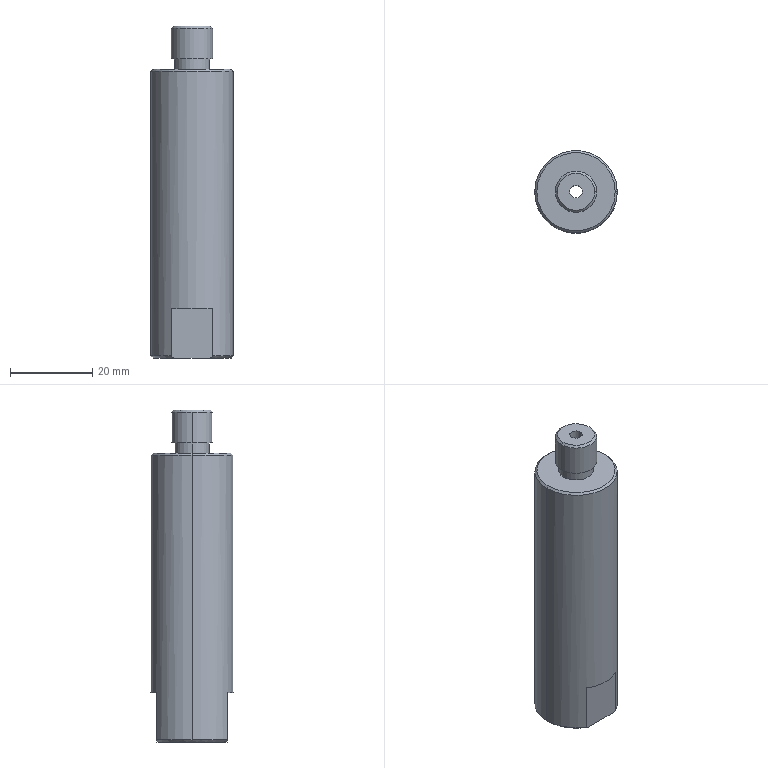Part | SolidWorks | features ICE 3, HoleWzd 2, Chamfer 1, Extrusion 1, MirrorPattern 1, RevCut 1 | 1 solid | 37 faces | box 20 x 20 x 80.5 mm | volume 19122 mm3 | plane 14 | cylinder 12 | cone 11 | commonest cylinder face diameters 3 x2 6 x2 8.5 x2 10 x2 11.125 x2 20 x2
STEP:
#1=CARTESIAN_POINT('',(4.5,0.,80.5));
#2=VERTEX_POINT('',#1);
#3=CARTESIAN_POINT('',(-4.5,0.,80.5));
#4=VERTEX_POINT('',#3);
#5=CARTESIAN_POINT('',(0.,0.,80.5));
#6=DIRECTION('',(0.,0.,1.));
#7=DIRECTION('',(1.,0.,0.));
#8=AXIS2_PLACEMENT_3D('',#5,#6,#7);
#9=CIRCLE('',#8,4.5);
#10=EDGE_CURVE('',#2,#4,#9,.T.);
#11=ORIENTED_EDGE('',*,*,#10,.F.);
#12=CARTESIAN_POINT('',(5.,0.,80.));
#13=VERTEX_POINT('',#12);
#14=CARTESIAN_POINT('',(4.5,0.,80.5));
#15=DIRECTION('',(0.7071,0.,-0.7071));
#16=VECTOR('',#15,1000.);
#17=LINE('',#14,#16);
#18=EDGE_CURVE('',#2,#13,#17,.T.);
#19=ORIENTED_EDGE('',*,*,#18,.T.);
#20=CARTESIAN_POINT('',(-5.,0.,80.));
#21=VERTEX_POINT('',#20);
#22=CARTESIAN_POINT('',(0.,0.,80.));
#23=DIRECTION('',(0.,0.,-1.));
#24=DIRECTION('',(1.,0.,0.));
#25=AXIS2_PLACEMENT_3D('',#22,#23,#24);
#26=CIRCLE('',#25,5.);
#27=EDGE_CURVE('',#21,#13,#26,.T.);
#28=ORIENTED_EDGE('',*,*,#27,.F.);
#29=CARTESIAN_POINT('',(-4.5,0.,80.5));
#30=DIRECTION('',(-0.7071,0.,-0.7071));
#31=VECTOR('',#30,1000.);
#32=LINE('',#29,#31);
#33=EDGE_CURVE('',#4,#21,#32,.T.);
#34=ORIENTED_EDGE('',*,*,#33,.F.);
#35=EDGE_LOOP('',(#11,#19,#28,#34));
#36=FACE_OUTER_BOUND('',#35,.T.);
#37=CARTESIAN_POINT('',(0.,0.,80.5));
#38=DIRECTION('',(0.,0.,-1.));
#39=DIRECTION('',(-1.,0.,0.));
#40=AXIS2_PLACEMENT_3D('',#37,#38,#39);
#41=CONICAL_SURFACE('',#40,4.5,0.7854);
#42=ADVANCED_FACE('',(#36),#41,.T.);
#43=CARTESIAN_POINT('',(9.5,0.,70.));
#44=VERTEX_POINT('',#43);
#45=CARTESIAN_POINT('',(-9.5,0.,70.));
#46=VERTEX_POINT('',#45);
#47=CARTESIAN_POINT('',(0.,0.,70.));
#48=DIRECTION('',(0.,0.,1.));
#49=DIRECTION('',(1.,0.,0.));
#50=AXIS2_PLACEMENT_3D('',#47,#48,#49);
#51=CIRCLE('',#50,9.5);
#52=EDGE_CURVE('',#44,#46,#51,.T.);
#53=ORIENTED_EDGE('',*,*,#52,.F.);
#54=CARTESIAN_POINT('',(10.,0.,69.5));
#55=VERTEX_POINT('',#54);
#56=CARTESIAN_POINT('',(9.5,0.,70.));
#57=DIRECTION('',(0.7071,0.,-0.7071));
#58=VECTOR('',#57,1000.);
#59=LINE('',#56,#58);
#60=EDGE_CURVE('',#44,#55,#59,.T.);
#61=ORIENTED_EDGE('',*,*,#60,.T.);
#62=CARTESIAN_POINT('',(-10.,0.,69.5));
#63=VERTEX_POINT('',#62);
#64=CARTESIAN_POINT('',(0.,0.,69.5));
#65=DIRECTION('',(0.,0.,-1.));
#66=DIRECTION('',(1.,0.,0.));
#67=AXIS2_PLACEMENT_3D('',#64,#65,#66);
#68=CIRCLE('',#67,10.);
#69=EDGE_CURVE('',#63,#55,#68,.T.);
#70=ORIENTED_EDGE('',*,*,#69,.F.);
#71=CARTESIAN_POINT('',(-9.5,0.,70.));
#72=DIRECTION('',(-0.7071,0.,-0.7071));
#73=VECTOR('',#72,1000.);
#74=LINE('',#71,#73);
#75=EDGE_CURVE('',#46,#63,#74,.T.);
#76=ORIENTED_EDGE('',*,*,#75,.F.);
#77=EDGE_LOOP('',(#53,#61,#70,#76));
#78=FACE_OUTER_BOUND('',#77,.T.);
#79=CARTESIAN_POINT('',(0.,0.,70.));
#80=DIRECTION('',(0.,0.,-1.));
#81=DIRECTION('',(-1.,0.,0.));
#82=AXIS2_PLACEMENT_3D('',#79,#80,#81);
#83=CONICAL_SURFACE('',#82,9.5,0.7854);
#84=ADVANCED_FACE('',(#78),#83,.T.);
#85=CARTESIAN_POINT('',(-3.,0.,18.61));
#86=VERTEX_POINT('',#85);
#87=CARTESIAN_POINT('',(3.,0.,18.61));
#88=VERTEX_POINT('',#87);
#89=CARTESIAN_POINT('',(0.,0.,18.61));
#90=DIRECTION('',(0.,0.,1.));
#91=DIRECTION('',(-1.,0.,0.));
#92=AXIS2_PLACEMENT_3D('',#89,#90,#91);
#93=CIRCLE('',#92,3.);
#94=EDGE_CURVE('',#86,#88,#93,.T.);
#95=ORIENTED_EDGE('',*,*,#94,.F.);
#96=CARTESIAN_POINT('',(-3.,0.,65.));
#97=VERTEX_POINT('',#96);
#98=CARTESIAN_POINT('',(-3.,0.,65.));
#99=DIRECTION('',(0.,0.,1.));
#100=VECTOR('',#99,1000.);
#101=LINE('',#98,#100);
#102=EDGE_CURVE('',#86,#97,#101,.T.);
#103=ORIENTED_EDGE('',*,*,#102,.T.);
#104=CARTESIAN_POINT('',(3.,0.,65.));
#105=VERTEX_POINT('',#104);
#106=CARTESIAN_POINT('',(0.,0.,65.));
#107=DIRECTION('',(0.,0.,1.));
#108=DIRECTION('',(1.,0.,0.));
#109=AXIS2_PLACEMENT_3D('',#106,#107,#108);
#110=CIRCLE('',#109,3.);
#111=EDGE_CURVE('',#97,#105,#110,.T.);
#112=ORIENTED_EDGE('',*,*,#111,.T.);
#113=CARTESIAN_POINT('',(3.,0.,65.));
#114=DIRECTION('',(0.,0.,1.));
#115=VECTOR('',#114,1000.);
#116=LINE('',#113,#115);
#117=EDGE_CURVE('',#88,#105,#116,.T.);
#118=ORIENTED_EDGE('',*,*,#117,.F.);
#119=EDGE_LOOP('',(#95,#103,#112,#118));
#120=FACE_OUTER_BOUND('',#119,.T.);
#121=CARTESIAN_POINT('',(0.,0.,65.));
#122=DIRECTION('',(0.,0.,1.));
#123=DIRECTION('',(1.,0.,0.));
#124=AXIS2_PLACEMENT_3D('',#121,#122,#123);
#125=CYLINDRICAL_SURFACE('',#124,3.);
#126=ADVANCED_FACE('',(#120),#125,.F.);
#127=CARTESIAN_POINT('',(5.944,0.,10.02));
#128=VERTEX_POINT('',#127);
#129=CARTESIAN_POINT('',(-5.944,0.,10.02));
#130=VERTEX_POINT('',#129);
#131=CARTESIAN_POINT('',(0.,0.,10.02));
#132=DIRECTION('',(0.,0.,-1.));
#133=DIRECTION('',(-1.,0.,0.));
#134=AXIS2_PLACEMENT_3D('',#131,#132,#133);
#135=CIRCLE('',#134,5.944);
#136=EDGE_CURVE('',#128,#130,#135,.T.);
#137=ORIENTED_EDGE('',*,*,#136,.F.);
#138=CARTESIAN_POINT('',(6.244,0.,0.));
#139=VERTEX_POINT('',#138);
#140=CARTESIAN_POINT('',(6.244,0.,0.));
#141=DIRECTION('',(0.02993,0.,-0.9996));
#142=VECTOR('',#141,1000.);
#143=LINE('',#140,#142);
#144=EDGE_CURVE('',#128,#139,#143,.T.);
#145=ORIENTED_EDGE('',*,*,#144,.T.);
#146=CARTESIAN_POINT('',(-6.244,0.,0.));
#147=VERTEX_POINT('',#146);
#148=CARTESIAN_POINT('',(0.,0.,0.));
#149=DIRECTION('',(0.,0.,-1.));
#150=DIRECTION('',(-1.,0.,0.));
#151=AXIS2_PLACEMENT_3D('',#148,#149,#150);
#152=CIRCLE('',#151,6.244);
#153=EDGE_CURVE('',#139,#147,#152,.T.);
#154=ORIENTED_EDGE('',*,*,#153,.T.);
#155=CARTESIAN_POINT('',(-6.244,0.,0.));
#156=DIRECTION('',(-0.02993,0.,-0.9996));
#157=VECTOR('',#156,1000.);
#158=LINE('',#155,#157);
#159=EDGE_CURVE('',#130,#147,#158,.T.);
#160=ORIENTED_EDGE('',*,*,#159,.F.);
#161=EDGE_LOOP('',(#137,#145,#154,#160));
#162=FACE_OUTER_BOUND('',#161,.T.);
#163=CARTESIAN_POINT('',(0.,0.,0.));
#164=DIRECTION('',(0.,0.,-1.));
#165=DIRECTION('',(-1.,0.,0.));
#166=AXIS2_PLACEMENT_3D('',#163,#164,#165);
#167=CONICAL_SURFACE('',#166,6.244,0.02993);
#168=ADVANCED_FACE('',(#162),#167,.F.);
#169=CARTESIAN_POINT('',(5.563,0.,17.07));
#170=VERTEX_POINT('',#169);
#171=CARTESIAN_POINT('',(-5.563,0.,17.07));
#172=VERTEX_POINT('',#171);
#173=CARTESIAN_POINT('',(0.,0.,17.07));
#174=DIRECTION('',(0.,0.,-1.));
#175=DIRECTION('',(-1.,0.,0.));
#176=AXIS2_PLACEMENT_3D('',#173,#174,#175);
#177=CIRCLE('',#176,5.563);
#178=EDGE_CURVE('',#170,#172,#177,.T.);
#179=ORIENTED_EDGE('',*,*,#178,.F.);
#180=CARTESIAN_POINT('',(5.563,0.,10.02));
#181=VERTEX_POINT('',#180);
#182=CARTESIAN_POINT('',(5.563,0.,0.));
#183=DIRECTION('',(0.,0.,-1.));
#184=VECTOR('',#183,1000.);
#185=LINE('',#182,#184);
#186=EDGE_CURVE('',#170,#181,#185,.T.);
#187=ORIENTED_EDGE('',*,*,#186,.T.);
#188=CARTESIAN_POINT('',(-5.563,0.,10.02));
#189=VERTEX_POINT('',#188);
#190=CARTESIAN_POINT('',(0.,0.,10.02));
#191=DIRECTION('',(0.,0.,-1.));
#192=DIRECTION('',(-1.,0.,0.));
#193=AXIS2_PLACEMENT_3D('',#190,#191,#192);
#194=CIRCLE('',#193,5.563);
#195=EDGE_CURVE('',#181,#189,#194,.T.);
#196=ORIENTED_EDGE('',*,*,#195,.T.);
#197=CARTESIAN_POINT('',(-5.563,0.,0.));
#198=DIRECTION('',(0.,0.,-1.));
#199=VECTOR('',#198,1000.);
#200=LINE('',#197,#199);
#201=EDGE_CURVE('',#172,#189,#200,.T.);
#202=ORIENTED_EDGE('',*,*,#201,.F.);
#203=EDGE_LOOP('',(#179,#187,#196,#202));
#204=FACE_OUTER_BOUND('',#203,.T.);
#205=CARTESIAN_POINT('',(0.,0.,0.));
#206=DIRECTION('',(0.,0.,-1.));
#207=DIRECTION('',(-1.,0.,0.));
#208=AXIS2_PLACEMENT_3D('',#205,#206,#207);
#209=CYLINDRICAL_SURFACE('',#208,5.563);
#210=ADVANCED_FACE('',(#204),#209,.F.);
#211=ORIENTED_EDGE('',*,*,#94,.T.);
#212=CARTESIAN_POINT('',(5.563,0.,17.07));
#213=DIRECTION('',(0.8572,0.,-0.515));
#214=VECTOR('',#213,1000.);
#215=LINE('',#212,#214);
#216=EDGE_CURVE('',#88,#170,#215,.T.);
#217=ORIENTED_EDGE('',*,*,#216,.T.);
#218=ORIENTED_EDGE('',*,*,#178,.T.);
#219=CARTESIAN_POINT('',(-5.563,0.,17.07));
#220=DIRECTION('',(-0.8572,0.,-0.515));
#221=VECTOR('',#220,1000.);
#222=LINE('',#219,#221);
#223=EDGE_CURVE('',#86,#172,#222,.T.);
#224=ORIENTED_EDGE('',*,*,#223,.F.);
#225=EDGE_LOOP('',(#211,#217,#218,#224));
#226=FACE_OUTER_BOUND('',#225,.T.);
#227=CARTESIAN_POINT('',(0.,0.,17.07));
#228=DIRECTION('',(0.,0.,-1.));
#229=DIRECTION('',(-1.,0.,0.));
#230=AXIS2_PLACEMENT_3D('',#227,#228,#229);
#231=CONICAL_SURFACE('',#230,5.563,1.03);
#232=ADVANCED_FACE('',(#226),#231,.F.);
#233=CARTESIAN_POINT('',(1.5,0.,65.));
#234=VERTEX_POINT('',#233);
#235=CARTESIAN_POINT('',(-1.5,0.,65.));
#236=VERTEX_POINT('',#235);
#237=CARTESIAN_POINT('',(0.,0.,65.));
#238=DIRECTION('',(0.,0.,-1.));
#239=DIRECTION('',(1.,0.,0.));
#240=AXIS2_PLACEMENT_3D('',#237,#238,#239);
#241=CIRCLE('',#240,1.5);
#242=EDGE_CURVE('',#234,#236,#241,.T.);
#243=ORIENTED_EDGE('',*,*,#242,.T.);
#244=CARTESIAN_POINT('',(-1.5,0.,80.5));
#245=VERTEX_POINT('',#244);
#246=CARTESIAN_POINT('',(-1.5,0.,65.));
#247=DIRECTION('',(0.,0.,1.));
#248=VECTOR('',#247,1000.);
#249=LINE('',#246,#248);
#250=EDGE_CURVE('',#236,#245,#249,.T.);
#251=ORIENTED_EDGE('',*,*,#250,.T.);
#252=CARTESIAN_POINT('',(1.5,0.,80.5));
#253=VERTEX_POINT('',#252);
#254=CARTESIAN_POINT('',(0.,0.,80.5));
#255=DIRECTION('',(0.,0.,1.));
#256=DIRECTION('',(1.,0.,0.));
#257=AXIS2_PLACEMENT_3D('',#254,#255,#256);
#258=CIRCLE('',#257,1.5);
#259=EDGE_CURVE('',#245,#253,#258,.T.);
#260=ORIENTED_EDGE('',*,*,#259,.T.);
#261=CARTESIAN_POINT('',(1.5,0.,65.));
#262=DIRECTION('',(0.,0.,1.));
#263=VECTOR('',#262,1000.);
#264=LINE('',#261,#263);
#265=EDGE_CURVE('',#234,#253,#264,.T.);
#266=ORIENTED_EDGE('',*,*,#265,.F.);
#267=EDGE_LOOP('',(#243,#251,#260,#266));
#268=FACE_OUTER_BOUND('',#267,.T.);
#269=CARTESIAN_POINT('',(0.,0.,65.));
#270=DIRECTION('',(0.,0.,1.));
#271=DIRECTION('',(1.,0.,0.));
#272=AXIS2_PLACEMENT_3D('',#269,#270,#271);
#273=CYLINDRICAL_SURFACE('',#272,1.5);
#274=ADVANCED_FACE('',(#268),#273,.F.);
#275=ORIENTED_EDGE('',*,*,#27,.T.);
#276=CARTESIAN_POINT('',(5.,0.,72.5));
#277=VERTEX_POINT('',#276);
#278=CARTESIAN_POINT('',(5.,0.,80.5));
#279=DIRECTION('',(0.,0.,-1.));
#280=VECTOR('',#279,1000.);
#281=LINE('',#278,#280);
#282=EDGE_CURVE('',#13,#277,#281,.T.);
#283=ORIENTED_EDGE('',*,*,#282,.T.);
#284=CARTESIAN_POINT('',(-5.,0.,72.5));
#285=VERTEX_POINT('',#284);
#286=CARTESIAN_POINT('',(0.,0.,72.5));
#287=DIRECTION('',(0.,0.,1.));
#288=DIRECTION('',(1.,0.,0.));
#289=AXIS2_PLACEMENT_3D('',#286,#287,#288);
#290=CIRCLE('',#289,5.);
#291=EDGE_CURVE('',#277,#285,#290,.T.);
#292=ORIENTED_EDGE('',*,*,#291,.T.);
#293=CARTESIAN_POINT('',(-5.,0.,80.5));
#294=DIRECTION('',(0.,0.,-1.));
#295=VECTOR('',#294,1000.);
#296=LINE('',#293,#295);
#297=EDGE_CURVE('',#21,#285,#296,.T.);
#298=ORIENTED_EDGE('',*,*,#297,.F.);
#299=EDGE_LOOP('',(#275,#283,#292,#298));
#300=FACE_OUTER_BOUND('',#299,.T.);
#301=CARTESIAN_POINT('',(0.,0.,80.5));
#302=DIRECTION('',(0.,0.,-1.));
#303=DIRECTION('',(-1.,0.,0.));
#304=AXIS2_PLACEMENT_3D('',#301,#302,#303);
#305=CYLINDRICAL_SURFACE('',#304,5.);
#306=ADVANCED_FACE('',(#300),#305,.T.);
#307=CARTESIAN_POINT('',(4.25,0.,70.));
#308=VERTEX_POINT('',#307);
#309=CARTESIAN_POINT('',(-4.25,0.,70.));
#310=VERTEX_POINT('',#309);
#311=CARTESIAN_POINT('',(0.,0.,70.));
#312=DIRECTION('',(0.,0.,1.));
#313=DIRECTION('',(1.,0.,0.));
#314=AXIS2_PLACEMENT_3D('',#311,#312,#313);
#315=CIRCLE('',#314,4.25);
#316=EDGE_CURVE('',#308,#310,#315,.T.);
#317=ORIENTED_EDGE('',*,*,#316,.T.);
#318=CARTESIAN_POINT('',(-4.25,0.,72.5));
#319=VERTEX_POINT('',#318);
#320=CARTESIAN_POINT('',(-4.25,0.,80.5));
#321=DIRECTION('',(0.,0.,1.));
#322=VECTOR('',#321,1000.);
#323=LINE('',#320,#322);
#324=EDGE_CURVE('',#310,#319,#323,.T.);
#325=ORIENTED_EDGE('',*,*,#324,.T.);
#326=CARTESIAN_POINT('',(4.25,0.,72.5));
#327=VERTEX_POINT('',#326);
#328=CARTESIAN_POINT('',(0.,0.,72.5));
#329=DIRECTION('',(0.,0.,1.));
#330=DIRECTION('',(1.,0.,0.));
#331=AXIS2_PLACEMENT_3D('',#328,#329,#330);
#332=CIRCLE('',#331,4.25);
#333=EDGE_CURVE('',#327,#319,#332,.T.);
#334=ORIENTED_EDGE('',*,*,#333,.F.);
#335=CARTESIAN_POINT('',(4.25,0.,80.5));
#336=DIRECTION('',(0.,0.,1.));
#337=VECTOR('',#336,1000.);
#338=LINE('',#335,#337);
#339=EDGE_CURVE('',#308,#327,#338,.T.);
#340=ORIENTED_EDGE('',*,*,#339,.F.);
#341=EDGE_LOOP('',(#317,#325,#334,#340));
#342=FACE_OUTER_BOUND('',#341,.T.);
#343=CARTESIAN_POINT('',(0.,0.,80.5));
#344=DIRECTION('',(0.,0.,1.));
#345=DIRECTION('',(1.,0.,0.));
#346=AXIS2_PLACEMENT_3D('',#343,#344,#345);
#347=CYLINDRICAL_SURFACE('',#346,4.25);
#348=ADVANCED_FACE('',(#342),#347,.T.);
#349=CARTESIAN_POINT('',(9.5,0.,0.));
#350=VERTEX_POINT('',#349);
#351=CARTESIAN_POINT('',(4.243,-8.5,0.));
#352=VERTEX_POINT('',#351);
#353=CARTESIAN_POINT('',(0.,0.,0.));
#354=DIRECTION('',(0.,0.,-1.));
#355=DIRECTION('',(1.,0.,0.));
#356=AXIS2_PLACEMENT_3D('',#353,#354,#355);
#357=CIRCLE('',#356,9.5);
#358=EDGE_CURVE('',#350,#352,#357,.T.);
#359=ORIENTED_EDGE('',*,*,#358,.F.);
#360=CARTESIAN_POINT('',(10.,0.,0.5));
#361=VERTEX_POINT('',#360);
#362=CARTESIAN_POINT('',(10.,0.,0.5));
#363=DIRECTION('',(0.7071,0.,0.7071));
#364=VECTOR('',#363,1000.);
#365=LINE('',#362,#364);
#366=EDGE_CURVE('',#350,#361,#365,.T.);
#367=ORIENTED_EDGE('',*,*,#366,.T.);
#368=CARTESIAN_POINT('',(5.,-8.66,0.5));
#369=VERTEX_POINT('',#368);
#370=CARTESIAN_POINT('',(0.,0.,0.5));
#371=DIRECTION('',(0.,0.,1.));
#372=DIRECTION('',(1.,0.,0.));
#373=AXIS2_PLACEMENT_3D('',#370,#371,#372);
#374=CIRCLE('',#373,10.);
#375=EDGE_CURVE('',#369,#361,#374,.T.);
#376=ORIENTED_EDGE('',*,*,#375,.F.);
#377=CARTESIAN_POINT('',(5.,-8.5,0.3615));
#378=VERTEX_POINT('',#377);
#379=CARTESIAN_POINT('',(5.,-8.66,0.5));
#380=CARTESIAN_POINT('',(5.,-8.607,0.4538));
#381=CARTESIAN_POINT('',(5.,-8.553,0.4076));
#382=CARTESIAN_POINT('',(5.,-8.5,0.3615));
#383=B_SPLINE_CURVE_WITH_KNOTS('',3,(#379,#380,#381,#382),.UNSPECIFIED.,.F.,.F.,(4,4),(0.002946,0.003158),.UNSPECIFIED.);
#384=EDGE_CURVE('',#369,#378,#383,.T.);
#385=ORIENTED_EDGE('',*,*,#384,.T.);
#386=CARTESIAN_POINT('',(5.,-8.5,0.3615));
#387=CARTESIAN_POINT('',(4.751,-8.5,0.2351));
#388=CARTESIAN_POINT('',(4.498,-8.5,0.1139));
#389=CARTESIAN_POINT('',(4.243,-8.5,0.));
#390=B_SPLINE_CURVE_WITH_KNOTS('',3,(#386,#387,#388,#389),.UNSPECIFIED.,.F.,.F.,(4,4),(0.007243,0.008076),.UNSPECIFIED.);
#391=EDGE_CURVE('',#378,#352,#390,.T.);
#392=ORIENTED_EDGE('',*,*,#391,.T.);
#393=EDGE_LOOP('',(#359,#367,#376,#385,#392));
#394=FACE_OUTER_BOUND('',#393,.T.);
#395=CARTESIAN_POINT('',(0.,0.,0.5));
#396=DIRECTION('',(0.,0.,1.));
#397=DIRECTION('',(1.,0.,0.));
#398=AXIS2_PLACEMENT_3D('',#395,#396,#397);
#399=CONICAL_SURFACE('',#398,10.,0.7854);
#400=ADVANCED_FACE('',(#394),#399,.T.);
#401=ORIENTED_EDGE('',*,*,#69,.T.);
#402=CARTESIAN_POINT('',(10.,0.,70.));
#403=DIRECTION('',(0.,0.,-1.));
#404=VECTOR('',#403,1000.);
#405=LINE('',#402,#404);
#406=EDGE_CURVE('',#55,#361,#405,.T.);
#407=ORIENTED_EDGE('',*,*,#406,.T.);
#408=CARTESIAN_POINT('',(5.,8.66,0.5));
#409=VERTEX_POINT('',#408);
#410=CARTESIAN_POINT('',(0.,0.,0.5));
#411=DIRECTION('',(0.,0.,1.));
#412=DIRECTION('',(1.,0.,0.));
#413=AXIS2_PLACEMENT_3D('',#410,#411,#412);
#414=CIRCLE('',#413,10.);
#415=EDGE_CURVE('',#361,#409,#414,.T.);
#416=ORIENTED_EDGE('',*,*,#415,.T.);
#417=CARTESIAN_POINT('',(5.,8.66,12.));
#418=VERTEX_POINT('',#417);
#419=CARTESIAN_POINT('',(5.,8.66,70.));
#420=DIRECTION('',(0.,0.,1.));
#421=VECTOR('',#420,1000.);
#422=LINE('',#419,#421);
#423=EDGE_CURVE('',#409,#418,#422,.T.);
#424=ORIENTED_EDGE('',*,*,#423,.T.);
#425=CARTESIAN_POINT('',(-5.,8.66,12.));
#426=VERTEX_POINT('',#425);
#427=CARTESIAN_POINT('',(0.,0.,12.));
#428=DIRECTION('',(0.,0.,1.));
#429=DIRECTION('',(1.,0.,0.));
#430=AXIS2_PLACEMENT_3D('',#427,#428,#429);
#431=CIRCLE('',#430,10.);
#432=EDGE_CURVE('',#418,#426,#431,.T.);
#433=ORIENTED_EDGE('',*,*,#432,.T.);
#434=CARTESIAN_POINT('',(-5.,8.66,0.5));
#435=VERTEX_POINT('',#434);
#436=CARTESIAN_POINT('',(-5.,8.66,70.));
#437=DIRECTION('',(0.,0.,-1.));
#438=VECTOR('',#437,1000.);
#439=LINE('',#436,#438);
#440=EDGE_CURVE('',#426,#435,#439,.T.);
#441=ORIENTED_EDGE('',*,*,#440,.T.);
#442=CARTESIAN_POINT('',(-10.,0.,0.5));
#443=VERTEX_POINT('',#442);
#444=CARTESIAN_POINT('',(0.,0.,0.5));
#445=DIRECTION('',(0.,0.,1.));
#446=DIRECTION('',(1.,0.,0.));
#447=AXIS2_PLACEMENT_3D('',#444,#445,#446);
#448=CIRCLE('',#447,10.);
#449=EDGE_CURVE('',#435,#443,#448,.T.);
#450=ORIENTED_EDGE('',*,*,#449,.T.);
#451=CARTESIAN_POINT('',(-10.,0.,70.));
#452=DIRECTION('',(0.,0.,-1.));
#453=VECTOR('',#452,1000.);
#454=LINE('',#451,#453);
#455=EDGE_CURVE('',#63,#443,#454,.T.);
#456=ORIENTED_EDGE('',*,*,#455,.F.);
#457=EDGE_LOOP('',(#401,#407,#416,#424,#433,#441,#450,#456));
#458=FACE_OUTER_BOUND('',#457,.T.);
#459=CARTESIAN_POINT('',(0.,0.,70.));
#460=DIRECTION('',(0.,0.,-1.));
#461=DIRECTION('',(-1.,0.,0.));
#462=AXIS2_PLACEMENT_3D('',#459,#460,#461);
#463=CYLINDRICAL_SURFACE('',#462,10.);
#464=ADVANCED_FACE('',(#458),#463,.T.);
#465=CARTESIAN_POINT('',(0.,0.,0.));
#466=DIRECTION('',(0.,0.,-1.));
#467=DIRECTION('',(-1.,0.,0.));
#468=AXIS2_PLACEMENT_3D('',#465,#466,#467);
#469=CIRCLE('',#468,6.244);
#470=EDGE_CURVE('',#147,#139,#469,.T.);
#471=ORIENTED_EDGE('',*,*,#470,.F.);
#472=ORIENTED_EDGE('',*,*,#153,.F.);
#473=EDGE_LOOP('',(#471,#472));
#474=FACE_BOUND('',#473,.T.);
#475=CARTESIAN_POINT('',(-4.243,-8.5,0.));
#476=VERTEX_POINT('',#475);
#477=CARTESIAN_POINT('',(-5.,-8.5,0.));
#478=DIRECTION('',(-1.,0.,0.));
#479=VECTOR('',#478,1000.);
#480=LINE('',#477,#479);
#481=EDGE_CURVE('',#352,#476,#480,.T.);
#482=ORIENTED_EDGE('',*,*,#481,.T.);
#483=CARTESIAN_POINT('',(-4.243,8.5,0.));
#484=VERTEX_POINT('',#483);
#485=CARTESIAN_POINT('',(0.,0.,0.));
#486=DIRECTION('',(0.,0.,-1.));
#487=DIRECTION('',(1.,0.,0.));
#488=AXIS2_PLACEMENT_3D('',#485,#486,#487);
#489=CIRCLE('',#488,9.5);
#490=EDGE_CURVE('',#476,#484,#489,.T.);
#491=ORIENTED_EDGE('',*,*,#490,.T.);
#492=CARTESIAN_POINT('',(4.243,8.5,0.));
#493=VERTEX_POINT('',#492);
#494=CARTESIAN_POINT('',(-5.,8.5,0.));
#495=DIRECTION('',(-1.,0.,0.));
#496=VECTOR('',#495,1000.);
#497=LINE('',#494,#496);
#498=EDGE_CURVE('',#493,#484,#497,.T.);
#499=ORIENTED_EDGE('',*,*,#498,.F.);
#500=CARTESIAN_POINT('',(0.,0.,0.));
#501=DIRECTION('',(0.,0.,-1.));
#502=DIRECTION('',(1.,0.,0.));
#503=AXIS2_PLACEMENT_3D('',#500,#501,#502);
#504=CIRCLE('',#503,9.5);
#505=EDGE_CURVE('',#493,#350,#504,.T.);
#506=ORIENTED_EDGE('',*,*,#505,.T.);
#507=ORIENTED_EDGE('',*,*,#358,.T.);
#508=EDGE_LOOP('',(#482,#491,#499,#506,#507));
#509=FACE_OUTER_BOUND('',#508,.T.);
#510=CARTESIAN_POINT('',(0.,0.,0.));
#511=DIRECTION('',(0.,0.,1.));
#512=DIRECTION('',(1.,0.,0.));
#513=AXIS2_PLACEMENT_3D('',#510,#511,#512);
#514=PLANE('',#513);
#515=ADVANCED_FACE('',(#474,#509),#514,.F.);
#516=ORIENTED_EDGE('',*,*,#406,.F.);
#517=CARTESIAN_POINT('',(0.,0.,69.5));
#518=DIRECTION('',(0.,0.,-1.));
#519=DIRECTION('',(1.,0.,0.));
#520=AXIS2_PLACEMENT_3D('',#517,#518,#519);
#521=CIRCLE('',#520,10.);
#522=EDGE_CURVE('',#55,#63,#521,.T.);
#523=ORIENTED_EDGE('',*,*,#522,.T.);
#524=ORIENTED_EDGE('',*,*,#455,.T.);
#525=CARTESIAN_POINT('',(-5.,-8.66,0.5));
#526=VERTEX_POINT('',#525);
#527=CARTESIAN_POINT('',(0.,0.,0.5));
#528=DIRECTION('',(0.,0.,1.));
#529=DIRECTION('',(1.,0.,0.));
#530=AXIS2_PLACEMENT_3D('',#527,#528,#529);
#531=CIRCLE('',#530,10.);
#532=EDGE_CURVE('',#443,#526,#531,.T.);
#533=ORIENTED_EDGE('',*,*,#532,.T.);
#534=CARTESIAN_POINT('',(-5.,-8.66,12.));
#535=VERTEX_POINT('',#534);
#536=CARTESIAN_POINT('',(-5.,-8.66,70.));
#537=DIRECTION('',(0.,0.,-1.));
#538=VECTOR('',#537,1000.);
#539=LINE('',#536,#538);
#540=EDGE_CURVE('',#535,#526,#539,.T.);
#541=ORIENTED_EDGE('',*,*,#540,.F.);
#542=CARTESIAN_POINT('',(5.,-8.66,12.));
#543=VERTEX_POINT('',#542);
#544=CARTESIAN_POINT('',(0.,0.,12.));
#545=DIRECTION('',(0.,0.,-1.));
#546=DIRECTION('',(-1.,0.,0.));
#547=AXIS2_PLACEMENT_3D('',#544,#545,#546);
#548=CIRCLE('',#547,10.);
#549=EDGE_CURVE('',#543,#535,#548,.T.);
#550=ORIENTED_EDGE('',*,*,#549,.F.);
#551=CARTESIAN_POINT('',(5.,-8.66,70.));
#552=DIRECTION('',(0.,0.,1.));
#553=VECTOR('',#552,1000.);
#554=LINE('',#551,#553);
#555=EDGE_CURVE('',#369,#543,#554,.T.);
#556=ORIENTED_EDGE('',*,*,#555,.F.);
#557=ORIENTED_EDGE('',*,*,#375,.T.);
#558=EDGE_LOOP('',(#516,#523,#524,#533,#541,#550,#556,#557));
#559=FACE_OUTER_BOUND('',#558,.T.);
#560=CARTESIAN_POINT('',(0.,0.,70.));
#561=DIRECTION('',(0.,0.,-1.));
#562=DIRECTION('',(-1.,0.,0.));
#563=AXIS2_PLACEMENT_3D('',#560,#561,#562);
#564=CYLINDRICAL_SURFACE('',#563,10.);
#565=ADVANCED_FACE('',(#559),#564,.T.);
#566=ORIENTED_EDGE('',*,*,#366,.F.);
#567=ORIENTED_EDGE('',*,*,#505,.F.);
#568=CARTESIAN_POINT('',(5.,8.5,0.3615));
#569=VERTEX_POINT('',#568);
#570=CARTESIAN_POINT('',(4.243,8.5,0.));
#571=CARTESIAN_POINT('',(4.498,8.5,0.114));
#572=CARTESIAN_POINT('',(4.75,8.5,0.2349));
#573=CARTESIAN_POINT('',(5.,8.5,0.3615));
#574=B_SPLINE_CURVE_WITH_KNOTS('',3,(#570,#571,#572,#573),.UNSPECIFIED.,.F.,.F.,(4,4),(0.01684,0.01768),.UNSPECIFIED.);
#575=EDGE_CURVE('',#493,#569,#574,.T.);
#576=ORIENTED_EDGE('',*,*,#575,.T.);
#577=CARTESIAN_POINT('',(5.,8.66,0.5));
#578=CARTESIAN_POINT('',(5.,8.607,0.4538));
#579=CARTESIAN_POINT('',(5.,8.553,0.4076));
#580=CARTESIAN_POINT('',(5.,8.5,0.3615));
#581=B_SPLINE_CURVE_WITH_KNOTS('',3,(#577,#578,#579,#580),.UNSPECIFIED.,.F.,.F.,(4,4),(0.002946,0.003158),.UNSPECIFIED.);
#582=EDGE_CURVE('',#409,#569,#581,.T.);
#583=ORIENTED_EDGE('',*,*,#582,.F.);
#584=ORIENTED_EDGE('',*,*,#415,.F.);
#585=EDGE_LOOP('',(#566,#567,#576,#583,#584));
#586=FACE_OUTER_BOUND('',#585,.T.);
#587=CARTESIAN_POINT('',(0.,0.,0.5));
#588=DIRECTION('',(0.,0.,1.));
#589=DIRECTION('',(1.,0.,0.));
#590=AXIS2_PLACEMENT_3D('',#587,#588,#589);
#591=CONICAL_SURFACE('',#590,10.,0.7854);
#592=ADVANCED_FACE('',(#586),#591,.T.);
#593=CARTESIAN_POINT('',(-5.,-8.5,0.3615));
#594=VERTEX_POINT('',#593);
#595=CARTESIAN_POINT('',(-4.243,-8.5,0.));
#596=CARTESIAN_POINT('',(-4.498,-8.5,0.114));
#597=CARTESIAN_POINT('',(-4.75,-8.5,0.2349));
#598=CARTESIAN_POINT('',(-5.,-8.5,0.3615));
#599=B_SPLINE_CURVE_WITH_KNOTS('',3,(#595,#596,#597,#598),.UNSPECIFIED.,.F.,.F.,(4,4),(0.01684,0.01768),.UNSPECIFIED.);
#600=EDGE_CURVE('',#476,#594,#599,.T.);
#601=ORIENTED_EDGE('',*,*,#600,.T.);
#602=CARTESIAN_POINT('',(-5.,-8.5,0.3615));
#603=CARTESIAN_POINT('',(-5.,-8.553,0.4076));
#604=CARTESIAN_POINT('',(-5.,-8.607,0.4538));
#605=CARTESIAN_POINT('',(-5.,-8.66,0.5));
#606=B_SPLINE_CURVE_WITH_KNOTS('',3,(#602,#603,#604,#605),.UNSPECIFIED.,.F.,.F.,(4,4),(0.003021,0.003233),.UNSPECIFIED.);
#607=EDGE_CURVE('',#594,#526,#606,.T.);
#608=ORIENTED_EDGE('',*,*,#607,.T.);
#609=ORIENTED_EDGE('',*,*,#532,.F.);
#610=ORIENTED_EDGE('',*,*,#449,.F.);
#611=CARTESIAN_POINT('',(-5.,8.5,0.3615));
#612=VERTEX_POINT('',#611);
#613=CARTESIAN_POINT('',(-5.,8.5,0.3615));
#614=CARTESIAN_POINT('',(-5.,8.553,0.4076));
#615=CARTESIAN_POINT('',(-5.,8.607,0.4538));
#616=CARTESIAN_POINT('',(-5.,8.66,0.5));
#617=B_SPLINE_CURVE_WITH_KNOTS('',3,(#613,#614,#615,#616),.UNSPECIFIED.,.F.,.F.,(4,4),(0.003021,0.003233),.UNSPECIFIED.);
#618=EDGE_CURVE('',#612,#435,#617,.T.);
#619=ORIENTED_EDGE('',*,*,#618,.F.);
#620=CARTESIAN_POINT('',(-5.,8.5,0.3615));
#621=CARTESIAN_POINT('',(-4.751,8.5,0.2351));
#622=CARTESIAN_POINT('',(-4.498,8.5,0.1139));
#623=CARTESIAN_POINT('',(-4.243,8.5,0.));
#624=B_SPLINE_CURVE_WITH_KNOTS('',3,(#620,#621,#622,#623),.UNSPECIFIED.,.F.,.F.,(4,4),(0.007243,0.008076),.UNSPECIFIED.);
#625=EDGE_CURVE('',#612,#484,#624,.T.);
#626=ORIENTED_EDGE('',*,*,#625,.T.);
#627=ORIENTED_EDGE('',*,*,#490,.F.);
#628=EDGE_LOOP('',(#601,#608,#609,#610,#619,#626,#627));
#629=FACE_OUTER_BOUND('',#628,.T.);
#630=CARTESIAN_POINT('',(0.,0.,0.5));
#631=DIRECTION('',(0.,0.,1.));
#632=DIRECTION('',(1.,0.,0.));
#633=AXIS2_PLACEMENT_3D('',#630,#631,#632);
#634=CONICAL_SURFACE('',#633,10.,0.7854);
#635=ADVANCED_FACE('',(#629),#634,.T.);
#636=CARTESIAN_POINT('',(0.,0.,70.));
#637=DIRECTION('',(0.,0.,1.));
#638=DIRECTION('',(1.,0.,0.));
#639=AXIS2_PLACEMENT_3D('',#636,#637,#638);
#640=CIRCLE('',#639,9.5);
#641=EDGE_CURVE('',#46,#44,#640,.T.);
#642=ORIENTED_EDGE('',*,*,#641,.T.);
#643=ORIENTED_EDGE('',*,*,#52,.T.);
#644=EDGE_LOOP('',(#642,#643));
#645=FACE_OUTER_BOUND('',#644,.T.);
#646=ORIENTED_EDGE('',*,*,#316,.F.);
#647=CARTESIAN_POINT('',(0.,0.,70.));
#648=DIRECTION('',(0.,0.,1.));
#649=DIRECTION('',(1.,0.,0.));
#650=AXIS2_PLACEMENT_3D('',#647,#648,#649);
#651=CIRCLE('',#650,4.25);
#652=EDGE_CURVE('',#310,#308,#651,.T.);
#653=ORIENTED_EDGE('',*,*,#652,.F.);
#654=EDGE_LOOP('',(#646,#653));
#655=FACE_BOUND('',#654,.T.);
#656=CARTESIAN_POINT('',(0.,0.,70.));
#657=DIRECTION('',(0.,0.,1.));
#658=DIRECTION('',(1.,0.,0.));
#659=AXIS2_PLACEMENT_3D('',#656,#657,#658);
#660=PLANE('',#659);
#661=ADVANCED_FACE('',(#645,#655),#660,.T.);
#662=ORIENTED_EDGE('',*,*,#333,.T.);
#663=CARTESIAN_POINT('',(0.,0.,72.5));
#664=DIRECTION('',(0.,0.,1.));
#665=DIRECTION('',(1.,0.,0.));
#666=AXIS2_PLACEMENT_3D('',#663,#664,#665);
#667=CIRCLE('',#666,4.25);
#668=EDGE_CURVE('',#319,#327,#667,.T.);
#669=ORIENTED_EDGE('',*,*,#668,.T.);
#670=EDGE_LOOP('',(#662,#669));
#671=FACE_BOUND('',#670,.T.);
#672=CARTESIAN_POINT('',(0.,0.,72.5));
#673=DIRECTION('',(0.,0.,1.));
#674=DIRECTION('',(1.,0.,0.));
#675=AXIS2_PLACEMENT_3D('',#672,#673,#674);
#676=CIRCLE('',#675,5.);
#677=EDGE_CURVE('',#285,#277,#676,.T.);
#678=ORIENTED_EDGE('',*,*,#677,.F.);
#679=ORIENTED_EDGE('',*,*,#291,.F.);
#680=EDGE_LOOP('',(#678,#679));
#681=FACE_OUTER_BOUND('',#680,.T.);
#682=CARTESIAN_POINT('',(-5.,0.,72.5));
#683=DIRECTION('',(0.,0.,-1.));
#684=DIRECTION('',(-1.,0.,0.));
#685=AXIS2_PLACEMENT_3D('',#682,#683,#684);
#686=PLANE('',#685);
#687=ADVANCED_FACE('',(#671,#681),#686,.T.);
#688=ORIENTED_EDGE('',*,*,#324,.F.);
#689=ORIENTED_EDGE('',*,*,#652,.T.);
#690=ORIENTED_EDGE('',*,*,#339,.T.);
#691=ORIENTED_EDGE('',*,*,#668,.F.);
#692=EDGE_LOOP('',(#688,#689,#690,#691));
#693=FACE_OUTER_BOUND('',#692,.T.);
#694=CARTESIAN_POINT('',(0.,0.,80.5));
#695=DIRECTION('',(0.,0.,1.));
#696=DIRECTION('',(1.,0.,0.));
#697=AXIS2_PLACEMENT_3D('',#694,#695,#696);
#698=CYLINDRICAL_SURFACE('',#697,4.25);
#699=ADVANCED_FACE('',(#693),#698,.T.);
#700=CARTESIAN_POINT('',(0.,0.,80.5));
#701=DIRECTION('',(0.,0.,1.));
#702=DIRECTION('',(1.,0.,0.));
#703=AXIS2_PLACEMENT_3D('',#700,#701,#702);
#704=CIRCLE('',#703,4.5);
#705=EDGE_CURVE('',#4,#2,#704,.T.);
#706=ORIENTED_EDGE('',*,*,#705,.T.);
#707=ORIENTED_EDGE('',*,*,#10,.T.);
#708=EDGE_LOOP('',(#706,#707));
#709=FACE_OUTER_BOUND('',#708,.T.);
#710=CARTESIAN_POINT('',(0.,0.,80.5));
#711=DIRECTION('',(0.,0.,1.));
#712=DIRECTION('',(1.,0.,0.));
#713=AXIS2_PLACEMENT_3D('',#710,#711,#712);
#714=CIRCLE('',#713,1.5);
#715=EDGE_CURVE('',#253,#245,#714,.T.);
#716=ORIENTED_EDGE('',*,*,#715,.F.);
#717=ORIENTED_EDGE('',*,*,#259,.F.);
#718=EDGE_LOOP('',(#716,#717));
#719=FACE_BOUND('',#718,.T.);
#720=CARTESIAN_POINT('',(0.,0.,80.5));
#721=DIRECTION('',(0.,0.,1.));
#722=DIRECTION('',(1.,0.,0.));
#723=AXIS2_PLACEMENT_3D('',#720,#721,#722);
#724=PLANE('',#723);
#725=ADVANCED_FACE('',(#709,#719),#724,.T.);
#726=ORIENTED_EDGE('',*,*,#282,.F.);
#727=CARTESIAN_POINT('',(0.,0.,80.));
#728=DIRECTION('',(0.,0.,-1.));
#729=DIRECTION('',(1.,0.,0.));
#730=AXIS2_PLACEMENT_3D('',#727,#728,#729);
#731=CIRCLE('',#730,5.);
#732=EDGE_CURVE('',#13,#21,#731,.T.);
#733=ORIENTED_EDGE('',*,*,#732,.T.);
#734=ORIENTED_EDGE('',*,*,#297,.T.);
#735=ORIENTED_EDGE('',*,*,#677,.T.);
#736=EDGE_LOOP('',(#726,#733,#734,#735));
#737=FACE_OUTER_BOUND('',#736,.T.);
#738=CARTESIAN_POINT('',(0.,0.,80.5));
#739=DIRECTION('',(0.,0.,-1.));
#740=DIRECTION('',(-1.,0.,0.));
#741=AXIS2_PLACEMENT_3D('',#738,#739,#740);
#742=CYLINDRICAL_SURFACE('',#741,5.);
#743=ADVANCED_FACE('',(#737),#742,.T.);
#744=ORIENTED_EDGE('',*,*,#250,.F.);
#745=CARTESIAN_POINT('',(0.,0.,65.));
#746=DIRECTION('',(0.,0.,-1.));
#747=DIRECTION('',(1.,0.,0.));
#748=AXIS2_PLACEMENT_3D('',#745,#746,#747);
#749=CIRCLE('',#748,1.5);
#750=EDGE_CURVE('',#236,#234,#749,.T.);
#751=ORIENTED_EDGE('',*,*,#750,.T.);
#752=ORIENTED_EDGE('',*,*,#265,.T.);
#753=ORIENTED_EDGE('',*,*,#715,.T.);
#754=EDGE_LOOP('',(#744,#751,#752,#753));
#755=FACE_OUTER_BOUND('',#754,.T.);
#756=CARTESIAN_POINT('',(0.,0.,65.));
#757=DIRECTION('',(0.,0.,1.));
#758=DIRECTION('',(1.,0.,0.));
#759=AXIS2_PLACEMENT_3D('',#756,#757,#758);
#760=CYLINDRICAL_SURFACE('',#759,1.5);
#761=ADVANCED_FACE('',(#755),#760,.F.);
#762=ORIENTED_EDGE('',*,*,#216,.F.);
#763=CARTESIAN_POINT('',(0.,0.,18.61));
#764=DIRECTION('',(0.,0.,1.));
#765=DIRECTION('',(-1.,0.,0.));
#766=AXIS2_PLACEMENT_3D('',#763,#764,#765);
#767=CIRCLE('',#766,3.);
#768=EDGE_CURVE('',#88,#86,#767,.T.);
#769=ORIENTED_EDGE('',*,*,#768,.T.);
#770=ORIENTED_EDGE('',*,*,#223,.T.);
#771=CARTESIAN_POINT('',(0.,0.,17.07));
#772=DIRECTION('',(0.,0.,-1.));
#773=DIRECTION('',(-1.,0.,0.));
#774=AXIS2_PLACEMENT_3D('',#771,#772,#773);
#775=CIRCLE('',#774,5.563);
#776=EDGE_CURVE('',#172,#170,#775,.T.);
#777=ORIENTED_EDGE('',*,*,#776,.T.);
#778=EDGE_LOOP('',(#762,#769,#770,#777));
#779=FACE_OUTER_BOUND('',#778,.T.);
#780=CARTESIAN_POINT('',(0.,0.,17.07));
#781=DIRECTION('',(0.,0.,-1.));
#782=DIRECTION('',(-1.,0.,0.));
#783=AXIS2_PLACEMENT_3D('',#780,#781,#782);
#784=CONICAL_SURFACE('',#783,5.563,1.03);
#785=ADVANCED_FACE('',(#779),#784,.F.);
#786=ORIENTED_EDGE('',*,*,#186,.F.);
#787=ORIENTED_EDGE('',*,*,#776,.F.);
#788=ORIENTED_EDGE('',*,*,#201,.T.);
#789=CARTESIAN_POINT('',(0.,0.,10.02));
#790=DIRECTION('',(0.,0.,-1.));
#791=DIRECTION('',(-1.,0.,0.));
#792=AXIS2_PLACEMENT_3D('',#789,#790,#791);
#793=CIRCLE('',#792,5.563);
#794=EDGE_CURVE('',#189,#181,#793,.T.);
#795=ORIENTED_EDGE('',*,*,#794,.T.);
#796=EDGE_LOOP('',(#786,#787,#788,#795));
#797=FACE_OUTER_BOUND('',#796,.T.);
#798=CARTESIAN_POINT('',(0.,0.,0.));
#799=DIRECTION('',(0.,0.,-1.));
#800=DIRECTION('',(-1.,0.,0.));
#801=AXIS2_PLACEMENT_3D('',#798,#799,#800);
#802=CYLINDRICAL_SURFACE('',#801,5.563);
#803=ADVANCED_FACE('',(#797),#802,.F.);
#804=ORIENTED_EDGE('',*,*,#794,.F.);
#805=ORIENTED_EDGE('',*,*,#195,.F.);
#806=EDGE_LOOP('',(#804,#805));
#807=FACE_BOUND('',#806,.T.);
#808=CARTESIAN_POINT('',(0.,0.,10.02));
#809=DIRECTION('',(0.,0.,-1.));
#810=DIRECTION('',(-1.,0.,0.));
#811=AXIS2_PLACEMENT_3D('',#808,#809,#810);
#812=CIRCLE('',#811,5.944);
#813=EDGE_CURVE('',#130,#128,#812,.T.);
#814=ORIENTED_EDGE('',*,*,#813,.T.);
#815=ORIENTED_EDGE('',*,*,#136,.T.);
#816=EDGE_LOOP('',(#814,#815));
#817=FACE_OUTER_BOUND('',#816,.T.);
#818=CARTESIAN_POINT('',(5.563,0.,10.02));
#819=DIRECTION('',(0.,0.,1.));
#820=DIRECTION('',(1.,0.,0.));
#821=AXIS2_PLACEMENT_3D('',#818,#819,#820);
#822=PLANE('',#821);
#823=ADVANCED_FACE('',(#807,#817),#822,.F.);
#824=ORIENTED_EDGE('',*,*,#144,.F.);
#825=ORIENTED_EDGE('',*,*,#813,.F.);
#826=ORIENTED_EDGE('',*,*,#159,.T.);
#827=ORIENTED_EDGE('',*,*,#470,.T.);
#828=EDGE_LOOP('',(#824,#825,#826,#827));
#829=FACE_OUTER_BOUND('',#828,.T.);
#830=CARTESIAN_POINT('',(0.,0.,0.));
#831=DIRECTION('',(0.,0.,-1.));
#832=DIRECTION('',(-1.,0.,0.));
#833=AXIS2_PLACEMENT_3D('',#830,#831,#832);
#834=CONICAL_SURFACE('',#833,6.244,0.02993);
#835=ADVANCED_FACE('',(#829),#834,.F.);
#836=CARTESIAN_POINT('',(0.,0.,65.));
#837=DIRECTION('',(0.,0.,1.));
#838=DIRECTION('',(1.,0.,0.));
#839=AXIS2_PLACEMENT_3D('',#836,#837,#838);
#840=CIRCLE('',#839,3.);
#841=EDGE_CURVE('',#105,#97,#840,.T.);
#842=ORIENTED_EDGE('',*,*,#841,.F.);
#843=ORIENTED_EDGE('',*,*,#111,.F.);
#844=EDGE_LOOP('',(#842,#843));
#845=FACE_OUTER_BOUND('',#844,.T.);
#846=ORIENTED_EDGE('',*,*,#242,.F.);
#847=ORIENTED_EDGE('',*,*,#750,.F.);
#848=EDGE_LOOP('',(#846,#847));
#849=FACE_BOUND('',#848,.T.);
#850=CARTESIAN_POINT('',(3.,0.,65.));
#851=DIRECTION('',(0.,0.,1.));
#852=DIRECTION('',(1.,0.,0.));
#853=AXIS2_PLACEMENT_3D('',#850,#851,#852);
#854=PLANE('',#853);
#855=ADVANCED_FACE('',(#845,#849),#854,.F.);
#856=ORIENTED_EDGE('',*,*,#102,.F.);
#857=ORIENTED_EDGE('',*,*,#768,.F.);
#858=ORIENTED_EDGE('',*,*,#117,.T.);
#859=ORIENTED_EDGE('',*,*,#841,.T.);
#860=EDGE_LOOP('',(#856,#857,#858,#859));
#861=FACE_OUTER_BOUND('',#860,.T.);
#862=CARTESIAN_POINT('',(0.,0.,65.));
#863=DIRECTION('',(0.,0.,1.));
#864=DIRECTION('',(1.,0.,0.));
#865=AXIS2_PLACEMENT_3D('',#862,#863,#864);
#866=CYLINDRICAL_SURFACE('',#865,3.);
#867=ADVANCED_FACE('',(#861),#866,.F.);
#868=ORIENTED_EDGE('',*,*,#60,.F.);
#869=ORIENTED_EDGE('',*,*,#641,.F.);
#870=ORIENTED_EDGE('',*,*,#75,.T.);
#871=ORIENTED_EDGE('',*,*,#522,.F.);
#872=EDGE_LOOP('',(#868,#869,#870,#871));
#873=FACE_OUTER_BOUND('',#872,.T.);
#874=CARTESIAN_POINT('',(0.,0.,70.));
#875=DIRECTION('',(0.,0.,-1.));
#876=DIRECTION('',(-1.,0.,0.));
#877=AXIS2_PLACEMENT_3D('',#874,#875,#876);
#878=CONICAL_SURFACE('',#877,9.5,0.7854);
#879=ADVANCED_FACE('',(#873),#878,.T.);
#880=ORIENTED_EDGE('',*,*,#18,.F.);
#881=ORIENTED_EDGE('',*,*,#705,.F.);
#882=ORIENTED_EDGE('',*,*,#33,.T.);
#883=ORIENTED_EDGE('',*,*,#732,.F.);
#884=EDGE_LOOP('',(#880,#881,#882,#883));
#885=FACE_OUTER_BOUND('',#884,.T.);
#886=CARTESIAN_POINT('',(0.,0.,80.5));
#887=DIRECTION('',(0.,0.,-1.));
#888=DIRECTION('',(-1.,0.,0.));
#889=AXIS2_PLACEMENT_3D('',#886,#887,#888);
#890=CONICAL_SURFACE('',#889,4.5,0.7854);
#891=ADVANCED_FACE('',(#885),#890,.T.);
#892=CARTESIAN_POINT('',(5.,8.5,12.));
#893=VERTEX_POINT('',#892);
#894=CARTESIAN_POINT('',(5.,8.5,12.));
#895=DIRECTION('',(0.,1.,0.));
#896=VECTOR('',#895,1000.);
#897=LINE('',#894,#896);
#898=EDGE_CURVE('',#893,#418,#897,.T.);
#899=ORIENTED_EDGE('',*,*,#898,.F.);
#900=CARTESIAN_POINT('',(-5.,8.5,12.));
#901=VERTEX_POINT('',#900);
#902=CARTESIAN_POINT('',(-5.,8.5,12.));
#903=DIRECTION('',(1.,0.,0.));
#904=VECTOR('',#903,1000.);
#905=LINE('',#902,#904);
#906=EDGE_CURVE('',#901,#893,#905,.T.);
#907=ORIENTED_EDGE('',*,*,#906,.F.);
#908=CARTESIAN_POINT('',(-5.,8.5,12.));
#909=DIRECTION('',(0.,1.,0.));
#910=VECTOR('',#909,1000.);
#911=LINE('',#908,#910);
#912=EDGE_CURVE('',#901,#426,#911,.T.);
#913=ORIENTED_EDGE('',*,*,#912,.T.);
#914=ORIENTED_EDGE('',*,*,#432,.F.);
#915=EDGE_LOOP('',(#899,#907,#913,#914));
#916=FACE_OUTER_BOUND('',#915,.T.);
#917=CARTESIAN_POINT('',(-5.,8.5,12.));
#918=DIRECTION('',(0.,0.,1.));
#919=DIRECTION('',(1.,0.,0.));
#920=AXIS2_PLACEMENT_3D('',#917,#918,#919);
#921=PLANE('',#920);
#922=ADVANCED_FACE('',(#916),#921,.F.);
#923=ORIENTED_EDGE('',*,*,#912,.F.);
#924=CARTESIAN_POINT('',(-5.,8.5,0.));
#925=DIRECTION('',(0.,0.,1.));
#926=VECTOR('',#925,1000.);
#927=LINE('',#924,#926);
#928=EDGE_CURVE('',#612,#901,#927,.T.);
#929=ORIENTED_EDGE('',*,*,#928,.F.);
#930=ORIENTED_EDGE('',*,*,#618,.T.);
#931=ORIENTED_EDGE('',*,*,#440,.F.);
#932=EDGE_LOOP('',(#923,#929,#930,#931));
#933=FACE_OUTER_BOUND('',#932,.T.);
#934=CARTESIAN_POINT('',(-5.,8.5,0.));
#935=DIRECTION('',(-1.,0.,0.));
#936=DIRECTION('',(0.,0.,1.));
#937=AXIS2_PLACEMENT_3D('',#934,#935,#936);
#938=PLANE('',#937);
#939=ADVANCED_FACE('',(#933),#938,.F.);
#940=ORIENTED_EDGE('',*,*,#582,.T.);
#941=CARTESIAN_POINT('',(5.,8.5,0.));
#942=DIRECTION('',(0.,0.,-1.));
#943=VECTOR('',#942,1000.);
#944=LINE('',#941,#943);
#945=EDGE_CURVE('',#893,#569,#944,.T.);
#946=ORIENTED_EDGE('',*,*,#945,.F.);
#947=ORIENTED_EDGE('',*,*,#898,.T.);
#948=ORIENTED_EDGE('',*,*,#423,.F.);
#949=EDGE_LOOP('',(#940,#946,#947,#948));
#950=FACE_OUTER_BOUND('',#949,.T.);
#951=CARTESIAN_POINT('',(5.,8.5,0.));
#952=DIRECTION('',(1.,0.,0.));
#953=DIRECTION('',(0.,0.,-1.));
#954=AXIS2_PLACEMENT_3D('',#951,#952,#953);
#955=PLANE('',#954);
#956=ADVANCED_FACE('',(#950),#955,.F.);
#957=ORIENTED_EDGE('',*,*,#928,.T.);
#958=ORIENTED_EDGE('',*,*,#906,.T.);
#959=ORIENTED_EDGE('',*,*,#945,.T.);
#960=ORIENTED_EDGE('',*,*,#575,.F.);
#961=ORIENTED_EDGE('',*,*,#498,.T.);
#962=ORIENTED_EDGE('',*,*,#625,.F.);
#963=EDGE_LOOP('',(#957,#958,#959,#960,#961,#962));
#964=FACE_OUTER_BOUND('',#963,.T.);
#965=CARTESIAN_POINT('',(0.,8.5,0.));
#966=DIRECTION('',(0.,1.,0.));
#967=DIRECTION('',(0.,0.,1.));
#968=AXIS2_PLACEMENT_3D('',#965,#966,#967);
#969=PLANE('',#968);
#970=ADVANCED_FACE('',(#964),#969,.T.);
#971=CARTESIAN_POINT('',(5.,-8.5,12.));
#972=VERTEX_POINT('',#971);
#973=CARTESIAN_POINT('',(5.,-8.5,12.));
#974=DIRECTION('',(0.,-1.,0.));
#975=VECTOR('',#974,1000.);
#976=LINE('',#973,#975);
#977=EDGE_CURVE('',#972,#543,#976,.T.);
#978=ORIENTED_EDGE('',*,*,#977,.T.);
#979=ORIENTED_EDGE('',*,*,#549,.T.);
#980=CARTESIAN_POINT('',(-5.,-8.5,12.));
#981=VERTEX_POINT('',#980);
#982=CARTESIAN_POINT('',(-5.,-8.5,12.));
#983=DIRECTION('',(0.,-1.,0.));
#984=VECTOR('',#983,1000.);
#985=LINE('',#982,#984);
#986=EDGE_CURVE('',#981,#535,#985,.T.);
#987=ORIENTED_EDGE('',*,*,#986,.F.);
#988=CARTESIAN_POINT('',(-5.,-8.5,12.));
#989=DIRECTION('',(1.,0.,0.));
#990=VECTOR('',#989,1000.);
#991=LINE('',#988,#990);
#992=EDGE_CURVE('',#981,#972,#991,.T.);
#993=ORIENTED_EDGE('',*,*,#992,.T.);
#994=EDGE_LOOP('',(#978,#979,#987,#993));
#995=FACE_OUTER_BOUND('',#994,.T.);
#996=CARTESIAN_POINT('',(-5.,-8.5,12.));
#997=DIRECTION('',(0.,0.,-1.));
#998=DIRECTION('',(-1.,0.,0.));
#999=AXIS2_PLACEMENT_3D('',#996,#997,#998);
#1000=PLANE('',#999);
#1001=ADVANCED_FACE('',(#995),#1000,.T.);
#1002=ORIENTED_EDGE('',*,*,#540,.T.);
#1003=ORIENTED_EDGE('',*,*,#607,.F.);
#1004=CARTESIAN_POINT('',(-5.,-8.5,0.));
#1005=DIRECTION('',(0.,0.,1.));
#1006=VECTOR('',#1005,1000.);
#1007=LINE('',#1004,#1006);
#1008=EDGE_CURVE('',#594,#981,#1007,.T.);
#1009=ORIENTED_EDGE('',*,*,#1008,.T.);
#1010=ORIENTED_EDGE('',*,*,#986,.T.);
#1011=EDGE_LOOP('',(#1002,#1003,#1009,#1010));
#1012=FACE_OUTER_BOUND('',#1011,.T.);
#1013=CARTESIAN_POINT('',(-5.,-8.5,0.));
#1014=DIRECTION('',(1.,0.,0.));
#1015=DIRECTION('',(0.,0.,-1.));
#1016=AXIS2_PLACEMENT_3D('',#1013,#1014,#1015);
#1017=PLANE('',#1016);
#1018=ADVANCED_FACE('',(#1012),#1017,.T.);
#1019=ORIENTED_EDGE('',*,*,#555,.T.);
#1020=ORIENTED_EDGE('',*,*,#977,.F.);
#1021=CARTESIAN_POINT('',(5.,-8.5,0.));
#1022=DIRECTION('',(0.,0.,-1.));
#1023=VECTOR('',#1022,1000.);
#1024=LINE('',#1021,#1023);
#1025=EDGE_CURVE('',#972,#378,#1024,.T.);
#1026=ORIENTED_EDGE('',*,*,#1025,.T.);
#1027=ORIENTED_EDGE('',*,*,#384,.F.);
#1028=EDGE_LOOP('',(#1019,#1020,#1026,#1027));
#1029=FACE_OUTER_BOUND('',#1028,.T.);
#1030=CARTESIAN_POINT('',(5.,-8.5,0.));
#1031=DIRECTION('',(-1.,0.,0.));
#1032=DIRECTION('',(0.,0.,1.));
#1033=AXIS2_PLACEMENT_3D('',#1030,#1031,#1032);
#1034=PLANE('',#1033);
#1035=ADVANCED_FACE('',(#1029),#1034,.T.);
#1036=ORIENTED_EDGE('',*,*,#1025,.F.);
#1037=ORIENTED_EDGE('',*,*,#992,.F.);
#1038=ORIENTED_EDGE('',*,*,#1008,.F.);
#1039=ORIENTED_EDGE('',*,*,#600,.F.);
#1040=ORIENTED_EDGE('',*,*,#481,.F.);
#1041=ORIENTED_EDGE('',*,*,#391,.F.);
#1042=EDGE_LOOP('',(#1036,#1037,#1038,#1039,#1040,#1041));
#1043=FACE_OUTER_BOUND('',#1042,.T.);
#1044=CARTESIAN_POINT('',(0.,-8.5,0.));
#1045=DIRECTION('',(0.,-1.,0.));
#1046=DIRECTION('',(0.,0.,1.));
#1047=AXIS2_PLACEMENT_3D('',#1044,#1045,#1046);
#1048=PLANE('',#1047);
#1049=ADVANCED_FACE('',(#1043),#1048,.T.);
#1050=CLOSED_SHELL('',(#42,#84,#126,#168,#210,#232,#274,#306,#348,#400,#464,#515,#565,#592,#635,#661,#687,#699,#725,#743,#761,#785,#803,#823,#835,#855,#867,#879,#891,#922,#939,#956,#970,#1001,#1018,#1035,#1049));
#1051=MANIFOLD_SOLID_BREP('',#1050);
#1052=CARTESIAN_POINT('',(0.,0.,0.));
#1053=DIRECTION('',(0.,0.,1.));
#1054=DIRECTION('',(1.,0.,0.));
#1055=AXIS2_PLACEMENT_3D('',#1052,#1053,#1054);
#1056=(LENGTH_UNIT()NAMED_UNIT(*)SI_UNIT(.MILLI.,.METRE.));
#1057=UNCERTAINTY_MEASURE_WITH_UNIT(LENGTH_MEASURE(0.00001),#1056,'','');
#1058=(NAMED_UNIT(*)PLANE_ANGLE_UNIT()SI_UNIT($,.RADIAN.));
#1059=(NAMED_UNIT(*)SI_UNIT($,.STERADIAN.)SOLID_ANGLE_UNIT());
#1060=(GEOMETRIC_REPRESENTATION_CONTEXT(3)GLOBAL_UNCERTAINTY_ASSIGNED_CONTEXT((#1057))GLOBAL_UNIT_ASSIGNED_CONTEXT((#1056,#1058,#1059))REPRESENTATION_CONTEXT('',''));
#1061=ADVANCED_BREP_SHAPE_REPRESENTATION('',(#1051,#1055),#1060);